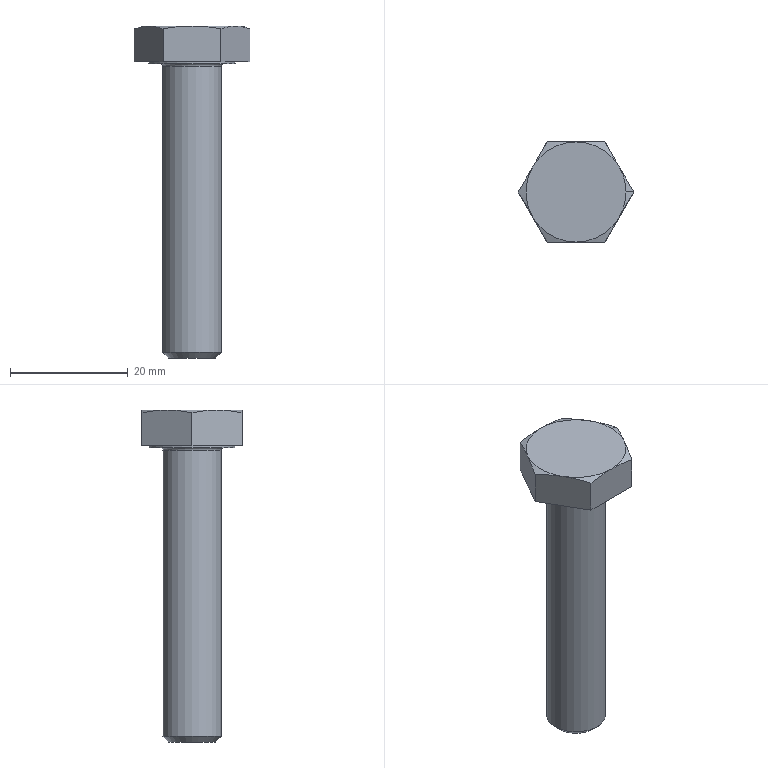Part | STEP file | Screw_set_M10x45 | 1 solid | 21 faces | box 19.63 x 17 x 56.4 mm | volume 5488 mm3 | plane 10 | cone 8 | cylinder 2 | torus 1 | commonest cylinder face diameters 10 x1 14.7 x1